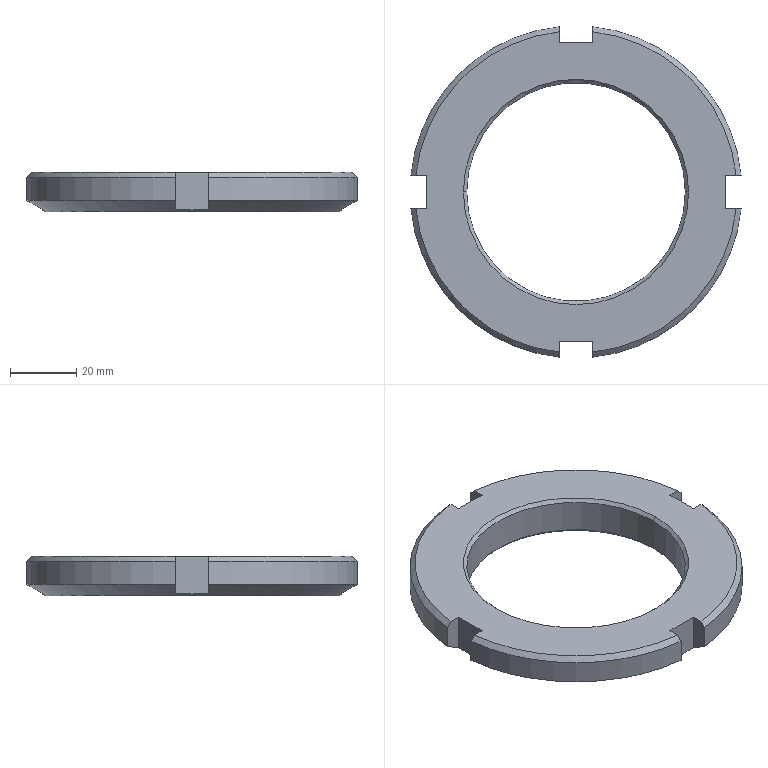Part | SolidWorks | features Chamfer 3, CirPattern 1, Cut 1, Extrusion 1 | 1 solid | 30 faces | box 99.499 x 99.499 x 12 mm | volume 47793 mm3 | plane 14 | cone 10 | cylinder 6 | commonest cylinder face diameters 100 x4 65.835 x2
STEP:
#1=CARTESIAN_POINT('',(-32.917,0.,11.));
#2=VERTEX_POINT('',#1);
#3=CARTESIAN_POINT('',(32.917,0.,11.));
#4=VERTEX_POINT('',#3);
#5=CARTESIAN_POINT('',(0.,0.,11.));
#6=DIRECTION('',(0.,0.,1.));
#7=DIRECTION('',(1.,0.,0.));
#8=AXIS2_PLACEMENT_3D('',#5,#6,#7);
#9=CIRCLE('',#8,32.917);
#10=EDGE_CURVE('',#2,#4,#9,.T.);
#11=ORIENTED_EDGE('',*,*,#10,.F.);
#12=CARTESIAN_POINT('',(-33.918,0.,12.));
#13=VERTEX_POINT('',#12);
#14=CARTESIAN_POINT('',(-32.917,0.,11.));
#15=DIRECTION('',(-0.7071,0.,0.7071));
#16=VECTOR('',#15,1000.);
#17=LINE('',#14,#16);
#18=EDGE_CURVE('',#2,#13,#17,.T.);
#19=ORIENTED_EDGE('',*,*,#18,.T.);
#20=CARTESIAN_POINT('',(33.918,0.,12.));
#21=VERTEX_POINT('',#20);
#22=CARTESIAN_POINT('',(0.,0.,12.));
#23=DIRECTION('',(0.,0.,-1.));
#24=DIRECTION('',(1.,0.,0.));
#25=AXIS2_PLACEMENT_3D('',#22,#23,#24);
#26=CIRCLE('',#25,33.918);
#27=EDGE_CURVE('',#21,#13,#26,.T.);
#28=ORIENTED_EDGE('',*,*,#27,.F.);
#29=CARTESIAN_POINT('',(32.917,0.,11.));
#30=DIRECTION('',(0.7071,0.,0.7071));
#31=VECTOR('',#30,1000.);
#32=LINE('',#29,#31);
#33=EDGE_CURVE('',#4,#21,#32,.T.);
#34=ORIENTED_EDGE('',*,*,#33,.F.);
#35=EDGE_LOOP('',(#11,#19,#28,#34));
#36=FACE_OUTER_BOUND('',#35,.T.);
#37=CARTESIAN_POINT('',(0.,0.,11.));
#38=DIRECTION('',(0.,0.,1.));
#39=DIRECTION('',(1.,0.,0.));
#40=AXIS2_PLACEMENT_3D('',#37,#38,#39);
#41=CONICAL_SURFACE('',#40,32.917,0.7854);
#42=ADVANCED_FACE('',(#36),#41,.F.);
#43=CARTESIAN_POINT('',(32.917,0.,1.));
#44=VERTEX_POINT('',#43);
#45=CARTESIAN_POINT('',(-32.917,0.,1.));
#46=VERTEX_POINT('',#45);
#47=CARTESIAN_POINT('',(0.,0.,1.));
#48=DIRECTION('',(0.,0.,-1.));
#49=DIRECTION('',(1.,0.,0.));
#50=AXIS2_PLACEMENT_3D('',#47,#48,#49);
#51=CIRCLE('',#50,32.917);
#52=EDGE_CURVE('',#44,#46,#51,.T.);
#53=ORIENTED_EDGE('',*,*,#52,.F.);
#54=CARTESIAN_POINT('',(33.918,0.,0.));
#55=VERTEX_POINT('',#54);
#56=CARTESIAN_POINT('',(33.918,0.,0.));
#57=DIRECTION('',(0.7071,0.,-0.7071));
#58=VECTOR('',#57,1000.);
#59=LINE('',#56,#58);
#60=EDGE_CURVE('',#44,#55,#59,.T.);
#61=ORIENTED_EDGE('',*,*,#60,.T.);
#62=CARTESIAN_POINT('',(-33.918,0.,0.));
#63=VERTEX_POINT('',#62);
#64=CARTESIAN_POINT('',(0.,0.,0.));
#65=DIRECTION('',(0.,0.,1.));
#66=DIRECTION('',(1.,0.,0.));
#67=AXIS2_PLACEMENT_3D('',#64,#65,#66);
#68=CIRCLE('',#67,33.918);
#69=EDGE_CURVE('',#63,#55,#68,.T.);
#70=ORIENTED_EDGE('',*,*,#69,.F.);
#71=CARTESIAN_POINT('',(-33.918,0.,0.));
#72=DIRECTION('',(-0.7071,0.,-0.7071));
#73=VECTOR('',#72,1000.);
#74=LINE('',#71,#73);
#75=EDGE_CURVE('',#46,#63,#74,.T.);
#76=ORIENTED_EDGE('',*,*,#75,.F.);
#77=EDGE_LOOP('',(#53,#61,#70,#76));
#78=FACE_OUTER_BOUND('',#77,.T.);
#79=CARTESIAN_POINT('',(0.,0.,0.));
#80=DIRECTION('',(0.,0.,-1.));
#81=DIRECTION('',(-1.,0.,0.));
#82=AXIS2_PLACEMENT_3D('',#79,#80,#81);
#83=CONICAL_SURFACE('',#82,33.918,0.7854);
#84=ADVANCED_FACE('',(#78),#83,.F.);
#85=CARTESIAN_POINT('',(-44.,0.,0.));
#86=VERTEX_POINT('',#85);
#87=CARTESIAN_POINT('',(44.,0.,0.));
#88=VERTEX_POINT('',#87);
#89=CARTESIAN_POINT('',(0.,0.,0.));
#90=DIRECTION('',(0.,0.,-1.));
#91=DIRECTION('',(1.,0.,0.));
#92=AXIS2_PLACEMENT_3D('',#89,#90,#91);
#93=CIRCLE('',#92,44.);
#94=EDGE_CURVE('',#86,#88,#93,.T.);
#95=ORIENTED_EDGE('',*,*,#94,.F.);
#96=CARTESIAN_POINT('',(-44.999,0.,0.577));
#97=VERTEX_POINT('',#96);
#98=CARTESIAN_POINT('',(-50.,0.,3.464));
#99=DIRECTION('',(-0.866,0.,0.5));
#100=VECTOR('',#99,1000.);
#101=LINE('',#98,#100);
#102=EDGE_CURVE('',#86,#97,#101,.T.);
#103=ORIENTED_EDGE('',*,*,#102,.T.);
#104=CARTESIAN_POINT('',(-44.999,5.,0.7369));
#105=VERTEX_POINT('',#104);
#106=CARTESIAN_POINT('',(-44.999,5.,0.7369));
#107=CARTESIAN_POINT('',(-44.999,3.338,0.6309));
#108=CARTESIAN_POINT('',(-44.999,1.671,0.577));
#109=CARTESIAN_POINT('',(-44.999,0.,0.577));
#110=B_SPLINE_CURVE_WITH_KNOTS('',3,(#106,#107,#108,#109),.UNSPECIFIED.,.F.,.F.,(4,4),(0.01219,0.01718),.UNSPECIFIED.);
#111=EDGE_CURVE('',#105,#97,#110,.T.);
#112=ORIENTED_EDGE('',*,*,#111,.F.);
#113=CARTESIAN_POINT('',(-49.749,5.,3.464));
#114=VERTEX_POINT('',#113);
#115=CARTESIAN_POINT('',(-49.749,5.,3.464));
#116=CARTESIAN_POINT('',(-49.476,5.,3.307));
#117=CARTESIAN_POINT('',(-49.202,5.,3.15));
#118=CARTESIAN_POINT('',(-48.929,5.,2.993));
#119=CARTESIAN_POINT('',(-47.619,5.,2.241));
#120=CARTESIAN_POINT('',(-46.309,5.,1.489));
#121=CARTESIAN_POINT('',(-44.999,5.,0.7369));
#122=B_SPLINE_CURVE_WITH_KNOTS('',3,(#115,#116,#117,#118,#119,#120,#121),.UNSPECIFIED.,.F.,.F.,(4,3,4),(0.01027,0.01122,0.01575),.UNSPECIFIED.);
#123=EDGE_CURVE('',#114,#105,#122,.T.);
#124=ORIENTED_EDGE('',*,*,#123,.F.);
#125=CARTESIAN_POINT('',(-5.,49.749,3.464));
#126=VERTEX_POINT('',#125);
#127=CARTESIAN_POINT('',(0.,0.,3.464));
#128=DIRECTION('',(0.,0.,1.));
#129=DIRECTION('',(1.,0.,0.));
#130=AXIS2_PLACEMENT_3D('',#127,#128,#129);
#131=CIRCLE('',#130,50.);
#132=EDGE_CURVE('',#126,#114,#131,.T.);
#133=ORIENTED_EDGE('',*,*,#132,.F.);
#134=CARTESIAN_POINT('',(-5.,44.999,0.7369));
#135=VERTEX_POINT('',#134);
#136=CARTESIAN_POINT('',(-5.,44.999,0.7369));
#137=CARTESIAN_POINT('',(-5.,45.167,0.833));
#138=CARTESIAN_POINT('',(-5.,45.334,0.9291));
#139=CARTESIAN_POINT('',(-5.,45.502,1.025));
#140=CARTESIAN_POINT('',(-5.,46.918,1.838));
#141=CARTESIAN_POINT('',(-5.,48.334,2.651));
#142=CARTESIAN_POINT('',(-5.,49.749,3.464));
#143=B_SPLINE_CURVE_WITH_KNOTS('',3,(#136,#137,#138,#139,#140,#141,#142),.UNSPECIFIED.,.F.,.F.,(4,3,4),(0.01064,0.01122,0.01612),.UNSPECIFIED.);
#144=EDGE_CURVE('',#135,#126,#143,.T.);
#145=ORIENTED_EDGE('',*,*,#144,.F.);
#146=CARTESIAN_POINT('',(5.,44.999,0.7369));
#147=VERTEX_POINT('',#146);
#148=CARTESIAN_POINT('',(5.,44.999,0.7369));
#149=CARTESIAN_POINT('',(3.342,44.999,0.6311));
#150=CARTESIAN_POINT('',(1.679,44.999,0.5772));
#151=CARTESIAN_POINT('',(-0.8215,44.999,0.5769));
#152=CARTESIAN_POINT('',(-1.656,44.999,0.5901));
#153=CARTESIAN_POINT('',(-3.328,44.999,0.6435));
#154=CARTESIAN_POINT('',(-4.165,44.999,0.6837));
#155=CARTESIAN_POINT('',(-5.,44.999,0.7369));
#156=B_SPLINE_CURVE_WITH_KNOTS('',3,(#148,#149,#150,#151,#152,#153,#154,#155),.UNSPECIFIED.,.F.,.F.,(4,2,2,4),(0.01219,0.01717,0.01966,0.02215),.UNSPECIFIED.);
#157=EDGE_CURVE('',#147,#135,#156,.T.);
#158=ORIENTED_EDGE('',*,*,#157,.F.);
#159=CARTESIAN_POINT('',(5.,49.749,3.464));
#160=VERTEX_POINT('',#159);
#161=CARTESIAN_POINT('',(5.,49.749,3.464));
#162=CARTESIAN_POINT('',(5.,48.334,2.651));
#163=CARTESIAN_POINT('',(5.,46.918,1.838));
#164=CARTESIAN_POINT('',(5.,45.502,1.025));
#165=CARTESIAN_POINT('',(5.,45.334,0.9291));
#166=CARTESIAN_POINT('',(5.,45.167,0.833));
#167=CARTESIAN_POINT('',(5.,44.999,0.7369));
#168=B_SPLINE_CURVE_WITH_KNOTS('',3,(#161,#162,#163,#164,#165,#166,#167),.UNSPECIFIED.,.F.,.F.,(4,3,4),(0.006321,0.01122,0.0118),.UNSPECIFIED.);
#169=EDGE_CURVE('',#160,#147,#168,.T.);
#170=ORIENTED_EDGE('',*,*,#169,.F.);
#171=CARTESIAN_POINT('',(49.749,5.,3.464));
#172=VERTEX_POINT('',#171);
#173=CARTESIAN_POINT('',(0.,0.,3.464));
#174=DIRECTION('',(0.,0.,1.));
#175=DIRECTION('',(1.,0.,0.));
#176=AXIS2_PLACEMENT_3D('',#173,#174,#175);
#177=CIRCLE('',#176,50.);
#178=EDGE_CURVE('',#172,#160,#177,.T.);
#179=ORIENTED_EDGE('',*,*,#178,.F.);
#180=CARTESIAN_POINT('',(44.999,5.,0.7369));
#181=VERTEX_POINT('',#180);
#182=CARTESIAN_POINT('',(44.999,5.,0.7369));
#183=CARTESIAN_POINT('',(45.167,5.,0.833));
#184=CARTESIAN_POINT('',(45.334,5.,0.9291));
#185=CARTESIAN_POINT('',(45.502,5.,1.025));
#186=CARTESIAN_POINT('',(46.918,5.,1.838));
#187=CARTESIAN_POINT('',(48.334,5.,2.651));
#188=CARTESIAN_POINT('',(49.749,5.,3.464));
#189=B_SPLINE_CURVE_WITH_KNOTS('',3,(#182,#183,#184,#185,#186,#187,#188),.UNSPECIFIED.,.F.,.F.,(4,3,4),(0.01064,0.01122,0.01612),.UNSPECIFIED.);
#190=EDGE_CURVE('',#181,#172,#189,.T.);
#191=ORIENTED_EDGE('',*,*,#190,.F.);
#192=CARTESIAN_POINT('',(44.999,0.,0.577));
#193=VERTEX_POINT('',#192);
#194=CARTESIAN_POINT('',(44.999,0.,0.577));
#195=CARTESIAN_POINT('',(44.999,1.671,0.577));
#196=CARTESIAN_POINT('',(44.999,3.338,0.6309));
#197=CARTESIAN_POINT('',(44.999,5.,0.7369));
#198=B_SPLINE_CURVE_WITH_KNOTS('',3,(#194,#195,#196,#197),.UNSPECIFIED.,.F.,.F.,(4,4),(0.02472,0.02972),.UNSPECIFIED.);
#199=EDGE_CURVE('',#193,#181,#198,.T.);
#200=ORIENTED_EDGE('',*,*,#199,.F.);
#201=CARTESIAN_POINT('',(50.,0.,3.464));
#202=DIRECTION('',(0.866,0.,0.5));
#203=VECTOR('',#202,1000.);
#204=LINE('',#201,#203);
#205=EDGE_CURVE('',#88,#193,#204,.T.);
#206=ORIENTED_EDGE('',*,*,#205,.F.);
#207=EDGE_LOOP('',(#95,#103,#112,#124,#133,#145,#158,#170,#179,#191,#200,#206));
#208=FACE_OUTER_BOUND('',#207,.T.);
#209=CARTESIAN_POINT('',(0.,0.,3.464));
#210=DIRECTION('',(0.,0.,1.));
#211=DIRECTION('',(1.,0.,0.));
#212=AXIS2_PLACEMENT_3D('',#209,#210,#211);
#213=CONICAL_SURFACE('',#212,50.,1.047);
#214=ADVANCED_FACE('',(#208),#213,.T.);
#215=ORIENTED_EDGE('',*,*,#10,.T.);
#216=CARTESIAN_POINT('',(32.917,0.,12.));
#217=DIRECTION('',(0.,0.,-1.));
#218=VECTOR('',#217,1000.);
#219=LINE('',#216,#218);
#220=EDGE_CURVE('',#4,#44,#219,.T.);
#221=ORIENTED_EDGE('',*,*,#220,.T.);
#222=ORIENTED_EDGE('',*,*,#52,.T.);
#223=CARTESIAN_POINT('',(-32.917,0.,12.));
#224=DIRECTION('',(0.,0.,-1.));
#225=VECTOR('',#224,1000.);
#226=LINE('',#223,#225);
#227=EDGE_CURVE('',#2,#46,#226,.T.);
#228=ORIENTED_EDGE('',*,*,#227,.F.);
#229=EDGE_LOOP('',(#215,#221,#222,#228));
#230=FACE_OUTER_BOUND('',#229,.T.);
#231=CARTESIAN_POINT('',(0.,0.,12.));
#232=DIRECTION('',(0.,0.,-1.));
#233=DIRECTION('',(-1.,0.,0.));
#234=AXIS2_PLACEMENT_3D('',#231,#232,#233);
#235=CYLINDRICAL_SURFACE('',#234,32.917);
#236=ADVANCED_FACE('',(#230),#235,.F.);
#237=CARTESIAN_POINT('',(5.,49.749,10.5));
#238=VERTEX_POINT('',#237);
#239=CARTESIAN_POINT('',(49.749,5.,10.5));
#240=VERTEX_POINT('',#239);
#241=CARTESIAN_POINT('',(0.,0.,10.5));
#242=DIRECTION('',(0.,0.,-1.));
#243=DIRECTION('',(1.,0.,0.));
#244=AXIS2_PLACEMENT_3D('',#241,#242,#243);
#245=CIRCLE('',#244,50.);
#246=EDGE_CURVE('',#238,#240,#245,.T.);
#247=ORIENTED_EDGE('',*,*,#246,.T.);
#248=CARTESIAN_POINT('',(49.749,5.,0.));
#249=DIRECTION('',(0.,0.,1.));
#250=VECTOR('',#249,1000.);
#251=LINE('',#248,#250);
#252=EDGE_CURVE('',#172,#240,#251,.T.);
#253=ORIENTED_EDGE('',*,*,#252,.F.);
#254=ORIENTED_EDGE('',*,*,#178,.T.);
#255=CARTESIAN_POINT('',(5.,49.749,0.));
#256=DIRECTION('',(0.,0.,1.));
#257=VECTOR('',#256,1000.);
#258=LINE('',#255,#257);
#259=EDGE_CURVE('',#160,#238,#258,.T.);
#260=ORIENTED_EDGE('',*,*,#259,.T.);
#261=EDGE_LOOP('',(#247,#253,#254,#260));
#262=FACE_OUTER_BOUND('',#261,.T.);
#263=CARTESIAN_POINT('',(0.,0.,12.));
#264=DIRECTION('',(0.,0.,-1.));
#265=DIRECTION('',(-1.,0.,0.));
#266=AXIS2_PLACEMENT_3D('',#263,#264,#265);
#267=CYLINDRICAL_SURFACE('',#266,50.);
#268=ADVANCED_FACE('',(#262),#267,.T.);
#269=CARTESIAN_POINT('',(48.242,5.,12.));
#270=VERTEX_POINT('',#269);
#271=CARTESIAN_POINT('',(49.749,5.,10.5));
#272=CARTESIAN_POINT('',(49.326,5.,10.921));
#273=CARTESIAN_POINT('',(48.903,5.,11.343));
#274=CARTESIAN_POINT('',(48.479,5.,11.764));
#275=CARTESIAN_POINT('',(48.4,5.,11.842));
#276=CARTESIAN_POINT('',(48.321,5.,11.921));
#277=CARTESIAN_POINT('',(48.242,5.,12.));
#278=B_SPLINE_CURVE_WITH_KNOTS('',3,(#271,#272,#273,#274,#275,#276,#277),.UNSPECIFIED.,.F.,.F.,(4,3,4),(0.00787,0.009662,0.009997),.UNSPECIFIED.);
#279=EDGE_CURVE('',#240,#270,#278,.T.);
#280=ORIENTED_EDGE('',*,*,#279,.F.);
#281=ORIENTED_EDGE('',*,*,#246,.F.);
#282=CARTESIAN_POINT('',(5.,48.242,12.));
#283=VERTEX_POINT('',#282);
#284=CARTESIAN_POINT('',(5.,48.242,12.));
#285=CARTESIAN_POINT('',(5.,48.321,11.921));
#286=CARTESIAN_POINT('',(5.,48.4,11.842));
#287=CARTESIAN_POINT('',(5.,48.479,11.764));
#288=CARTESIAN_POINT('',(5.,48.903,11.343));
#289=CARTESIAN_POINT('',(5.,49.326,10.921));
#290=CARTESIAN_POINT('',(5.,49.749,10.5));
#291=B_SPLINE_CURVE_WITH_KNOTS('',3,(#284,#285,#286,#287,#288,#289,#290),.UNSPECIFIED.,.F.,.F.,(4,3,4),(0.009327,0.009662,0.01145),.UNSPECIFIED.);
#292=EDGE_CURVE('',#283,#238,#291,.T.);
#293=ORIENTED_EDGE('',*,*,#292,.F.);
#294=CARTESIAN_POINT('',(0.,0.,12.));
#295=DIRECTION('',(0.,0.,1.));
#296=DIRECTION('',(1.,0.,0.));
#297=AXIS2_PLACEMENT_3D('',#294,#295,#296);
#298=CIRCLE('',#297,48.5);
#299=EDGE_CURVE('',#270,#283,#298,.T.);
#300=ORIENTED_EDGE('',*,*,#299,.F.);
#301=EDGE_LOOP('',(#280,#281,#293,#300));
#302=FACE_OUTER_BOUND('',#301,.T.);
#303=CARTESIAN_POINT('',(0.,0.,12.));
#304=DIRECTION('',(0.,0.,-1.));
#305=DIRECTION('',(-1.,0.,0.));
#306=AXIS2_PLACEMENT_3D('',#303,#304,#305);
#307=CONICAL_SURFACE('',#306,48.5,0.7854);
#308=ADVANCED_FACE('',(#302),#307,.T.);
#309=CARTESIAN_POINT('',(-49.749,5.,10.5));
#310=VERTEX_POINT('',#309);
#311=CARTESIAN_POINT('',(-5.,49.749,10.5));
#312=VERTEX_POINT('',#311);
#313=CARTESIAN_POINT('',(0.,0.,10.5));
#314=DIRECTION('',(0.,0.,-1.));
#315=DIRECTION('',(1.,0.,0.));
#316=AXIS2_PLACEMENT_3D('',#313,#314,#315);
#317=CIRCLE('',#316,50.);
#318=EDGE_CURVE('',#310,#312,#317,.T.);
#319=ORIENTED_EDGE('',*,*,#318,.T.);
#320=CARTESIAN_POINT('',(-5.,49.749,0.));
#321=DIRECTION('',(0.,0.,1.));
#322=VECTOR('',#321,1000.);
#323=LINE('',#320,#322);
#324=EDGE_CURVE('',#126,#312,#323,.T.);
#325=ORIENTED_EDGE('',*,*,#324,.F.);
#326=ORIENTED_EDGE('',*,*,#132,.T.);
#327=CARTESIAN_POINT('',(-49.749,5.,0.));
#328=DIRECTION('',(0.,0.,1.));
#329=VECTOR('',#328,1000.);
#330=LINE('',#327,#329);
#331=EDGE_CURVE('',#114,#310,#330,.T.);
#332=ORIENTED_EDGE('',*,*,#331,.T.);
#333=EDGE_LOOP('',(#319,#325,#326,#332));
#334=FACE_OUTER_BOUND('',#333,.T.);
#335=CARTESIAN_POINT('',(0.,0.,12.));
#336=DIRECTION('',(0.,0.,-1.));
#337=DIRECTION('',(-1.,0.,0.));
#338=AXIS2_PLACEMENT_3D('',#335,#336,#337);
#339=CYLINDRICAL_SURFACE('',#338,50.);
#340=ADVANCED_FACE('',(#334),#339,.T.);
#341=CARTESIAN_POINT('',(-5.,48.242,12.));
#342=VERTEX_POINT('',#341);
#343=CARTESIAN_POINT('',(-5.,49.749,10.5));
#344=CARTESIAN_POINT('',(-5.,49.326,10.921));
#345=CARTESIAN_POINT('',(-5.,48.903,11.343));
#346=CARTESIAN_POINT('',(-5.,48.479,11.764));
#347=CARTESIAN_POINT('',(-5.,48.4,11.842));
#348=CARTESIAN_POINT('',(-5.,48.321,11.921));
#349=CARTESIAN_POINT('',(-5.,48.242,12.));
#350=B_SPLINE_CURVE_WITH_KNOTS('',3,(#343,#344,#345,#346,#347,#348,#349),.UNSPECIFIED.,.F.,.F.,(4,3,4),(0.00787,0.009662,0.009997),.UNSPECIFIED.);
#351=EDGE_CURVE('',#312,#342,#350,.T.);
#352=ORIENTED_EDGE('',*,*,#351,.F.);
#353=ORIENTED_EDGE('',*,*,#318,.F.);
#354=CARTESIAN_POINT('',(-48.242,5.,12.));
#355=VERTEX_POINT('',#354);
#356=CARTESIAN_POINT('',(-48.242,5.,12.));
#357=CARTESIAN_POINT('',(-48.52,5.,11.723));
#358=CARTESIAN_POINT('',(-48.798,5.,11.447));
#359=CARTESIAN_POINT('',(-49.076,5.,11.17));
#360=CARTESIAN_POINT('',(-49.3,5.,10.947));
#361=CARTESIAN_POINT('',(-49.525,5.,10.723));
#362=CARTESIAN_POINT('',(-49.749,5.,10.5));
#363=B_SPLINE_CURVE_WITH_KNOTS('',3,(#356,#357,#358,#359,#360,#361,#362),.UNSPECIFIED.,.F.,.F.,(4,3,4),(0.008485,0.009662,0.01061),.UNSPECIFIED.);
#364=EDGE_CURVE('',#355,#310,#363,.T.);
#365=ORIENTED_EDGE('',*,*,#364,.F.);
#366=CARTESIAN_POINT('',(0.,0.,12.));
#367=DIRECTION('',(0.,0.,1.));
#368=DIRECTION('',(1.,0.,0.));
#369=AXIS2_PLACEMENT_3D('',#366,#367,#368);
#370=CIRCLE('',#369,48.5);
#371=EDGE_CURVE('',#342,#355,#370,.T.);
#372=ORIENTED_EDGE('',*,*,#371,.F.);
#373=EDGE_LOOP('',(#352,#353,#365,#372));
#374=FACE_OUTER_BOUND('',#373,.T.);
#375=CARTESIAN_POINT('',(0.,0.,12.));
#376=DIRECTION('',(0.,0.,-1.));
#377=DIRECTION('',(-1.,0.,0.));
#378=AXIS2_PLACEMENT_3D('',#375,#376,#377);
#379=CONICAL_SURFACE('',#378,48.5,0.7854);
#380=ADVANCED_FACE('',(#374),#379,.T.);
#381=CARTESIAN_POINT('',(-5.,-49.749,10.5));
#382=VERTEX_POINT('',#381);
#383=CARTESIAN_POINT('',(-49.749,-5.,10.5));
#384=VERTEX_POINT('',#383);
#385=CARTESIAN_POINT('',(0.,0.,10.5));
#386=DIRECTION('',(0.,0.,-1.));
#387=DIRECTION('',(1.,0.,0.));
#388=AXIS2_PLACEMENT_3D('',#385,#386,#387);
#389=CIRCLE('',#388,50.);
#390=EDGE_CURVE('',#382,#384,#389,.T.);
#391=ORIENTED_EDGE('',*,*,#390,.T.);
#392=CARTESIAN_POINT('',(-49.749,-5.,3.464));
#393=VERTEX_POINT('',#392);
#394=CARTESIAN_POINT('',(-49.749,-5.,0.));
#395=DIRECTION('',(0.,0.,1.));
#396=VECTOR('',#395,1000.);
#397=LINE('',#394,#396);
#398=EDGE_CURVE('',#393,#384,#397,.T.);
#399=ORIENTED_EDGE('',*,*,#398,.F.);
#400=CARTESIAN_POINT('',(-5.,-49.749,3.464));
#401=VERTEX_POINT('',#400);
#402=CARTESIAN_POINT('',(0.,0.,3.464));
#403=DIRECTION('',(0.,0.,1.));
#404=DIRECTION('',(1.,0.,0.));
#405=AXIS2_PLACEMENT_3D('',#402,#403,#404);
#406=CIRCLE('',#405,50.);
#407=EDGE_CURVE('',#393,#401,#406,.T.);
#408=ORIENTED_EDGE('',*,*,#407,.T.);
#409=CARTESIAN_POINT('',(-5.,-49.749,0.));
#410=DIRECTION('',(0.,0.,1.));
#411=VECTOR('',#410,1000.);
#412=LINE('',#409,#411);
#413=EDGE_CURVE('',#401,#382,#412,.T.);
#414=ORIENTED_EDGE('',*,*,#413,.T.);
#415=EDGE_LOOP('',(#391,#399,#408,#414));
#416=FACE_OUTER_BOUND('',#415,.T.);
#417=CARTESIAN_POINT('',(0.,0.,12.));
#418=DIRECTION('',(0.,0.,-1.));
#419=DIRECTION('',(-1.,0.,0.));
#420=AXIS2_PLACEMENT_3D('',#417,#418,#419);
#421=CYLINDRICAL_SURFACE('',#420,50.);
#422=ADVANCED_FACE('',(#416),#421,.T.);
#423=CARTESIAN_POINT('',(-48.242,-5.,12.));
#424=VERTEX_POINT('',#423);
#425=CARTESIAN_POINT('',(-49.749,-5.,10.5));
#426=CARTESIAN_POINT('',(-49.525,-5.,10.723));
#427=CARTESIAN_POINT('',(-49.3,-5.,10.947));
#428=CARTESIAN_POINT('',(-49.076,-5.,11.17));
#429=CARTESIAN_POINT('',(-48.798,-5.,11.447));
#430=CARTESIAN_POINT('',(-48.52,-5.,11.723));
#431=CARTESIAN_POINT('',(-48.242,-5.,12.));
#432=B_SPLINE_CURVE_WITH_KNOTS('',3,(#425,#426,#427,#428,#429,#430,#431),.UNSPECIFIED.,.F.,.F.,(4,3,4),(0.008712,0.009662,0.01084),.UNSPECIFIED.);
#433=EDGE_CURVE('',#384,#424,#432,.T.);
#434=ORIENTED_EDGE('',*,*,#433,.F.);
#435=ORIENTED_EDGE('',*,*,#390,.F.);
#436=CARTESIAN_POINT('',(-5.,-48.242,12.));
#437=VERTEX_POINT('',#436);
#438=CARTESIAN_POINT('',(-5.,-48.242,12.));
#439=CARTESIAN_POINT('',(-5.,-48.52,11.723));
#440=CARTESIAN_POINT('',(-5.,-48.798,11.447));
#441=CARTESIAN_POINT('',(-5.,-49.076,11.17));
#442=CARTESIAN_POINT('',(-5.,-49.3,10.947));
#443=CARTESIAN_POINT('',(-5.,-49.525,10.723));
#444=CARTESIAN_POINT('',(-5.,-49.749,10.5));
#445=B_SPLINE_CURVE_WITH_KNOTS('',3,(#438,#439,#440,#441,#442,#443,#444),.UNSPECIFIED.,.F.,.F.,(4,3,4),(0.008485,0.009662,0.01061),.UNSPECIFIED.);
#446=EDGE_CURVE('',#437,#382,#445,.T.);
#447=ORIENTED_EDGE('',*,*,#446,.F.);
#448=CARTESIAN_POINT('',(0.,0.,12.));
#449=DIRECTION('',(0.,0.,1.));
#450=DIRECTION('',(1.,0.,0.));
#451=AXIS2_PLACEMENT_3D('',#448,#449,#450);
#452=CIRCLE('',#451,48.5);
#453=EDGE_CURVE('',#424,#437,#452,.T.);
#454=ORIENTED_EDGE('',*,*,#453,.F.);
#455=EDGE_LOOP('',(#434,#435,#447,#454));
#456=FACE_OUTER_BOUND('',#455,.T.);
#457=CARTESIAN_POINT('',(0.,0.,12.));
#458=DIRECTION('',(0.,0.,-1.));
#459=DIRECTION('',(-1.,0.,0.));
#460=AXIS2_PLACEMENT_3D('',#457,#458,#459);
#461=CONICAL_SURFACE('',#460,48.5,0.7854);
#462=ADVANCED_FACE('',(#456),#461,.T.);
#463=ORIENTED_EDGE('',*,*,#27,.T.);
#464=CARTESIAN_POINT('',(0.,0.,12.));
#465=DIRECTION('',(0.,0.,-1.));
#466=DIRECTION('',(1.,0.,0.));
#467=AXIS2_PLACEMENT_3D('',#464,#465,#466);
#468=CIRCLE('',#467,33.918);
#469=EDGE_CURVE('',#13,#21,#468,.T.);
#470=ORIENTED_EDGE('',*,*,#469,.T.);
#471=EDGE_LOOP('',(#463,#470));
#472=FACE_BOUND('',#471,.T.);
#473=CARTESIAN_POINT('',(44.999,5.,12.));
#474=VERTEX_POINT('',#473);
#475=CARTESIAN_POINT('',(44.999,5.,12.));
#476=DIRECTION('',(-1.,0.,0.));
#477=VECTOR('',#476,1000.);
#478=LINE('',#475,#477);
#479=EDGE_CURVE('',#270,#474,#478,.T.);
#480=ORIENTED_EDGE('',*,*,#479,.F.);
#481=ORIENTED_EDGE('',*,*,#299,.T.);
#482=CARTESIAN_POINT('',(5.,44.999,12.));
#483=VERTEX_POINT('',#482);
#484=CARTESIAN_POINT('',(5.,44.999,12.));
#485=DIRECTION('',(0.,1.,0.));
#486=VECTOR('',#485,1000.);
#487=LINE('',#484,#486);
#488=EDGE_CURVE('',#483,#283,#487,.T.);
#489=ORIENTED_EDGE('',*,*,#488,.F.);
#490=CARTESIAN_POINT('',(-5.,44.999,12.));
#491=VERTEX_POINT('',#490);
#492=CARTESIAN_POINT('',(5.,44.999,12.));
#493=DIRECTION('',(1.,0.,0.));
#494=VECTOR('',#493,1000.);
#495=LINE('',#492,#494);
#496=EDGE_CURVE('',#491,#483,#495,.T.);
#497=ORIENTED_EDGE('',*,*,#496,.F.);
#498=CARTESIAN_POINT('',(-5.,44.999,12.));
#499=DIRECTION('',(0.,-1.,0.));
#500=VECTOR('',#499,1000.);
#501=LINE('',#498,#500);
#502=EDGE_CURVE('',#342,#491,#501,.T.);
#503=ORIENTED_EDGE('',*,*,#502,.F.);
#504=ORIENTED_EDGE('',*,*,#371,.T.);
#505=CARTESIAN_POINT('',(-44.999,5.,12.));
#506=VERTEX_POINT('',#505);
#507=CARTESIAN_POINT('',(-44.999,5.,12.));
#508=DIRECTION('',(-1.,0.,0.));
#509=VECTOR('',#508,1000.);
#510=LINE('',#507,#509);
#511=EDGE_CURVE('',#506,#355,#510,.T.);
#512=ORIENTED_EDGE('',*,*,#511,.F.);
#513=CARTESIAN_POINT('',(-44.999,-5.,12.));
#514=VERTEX_POINT('',#513);
#515=CARTESIAN_POINT('',(-44.999,5.,12.));
#516=DIRECTION('',(0.,1.,0.));
#517=VECTOR('',#516,1000.);
#518=LINE('',#515,#517);
#519=EDGE_CURVE('',#514,#506,#518,.T.);
#520=ORIENTED_EDGE('',*,*,#519,.F.);
#521=CARTESIAN_POINT('',(-44.999,-5.,12.));
#522=DIRECTION('',(1.,0.,0.));
#523=VECTOR('',#522,1000.);
#524=LINE('',#521,#523);
#525=EDGE_CURVE('',#424,#514,#524,.T.);
#526=ORIENTED_EDGE('',*,*,#525,.F.);
#527=ORIENTED_EDGE('',*,*,#453,.T.);
#528=CARTESIAN_POINT('',(-5.,-44.999,12.));
#529=VERTEX_POINT('',#528);
#530=CARTESIAN_POINT('',(-5.,-44.999,12.));
#531=DIRECTION('',(0.,-1.,0.));
#532=VECTOR('',#531,1000.);
#533=LINE('',#530,#532);
#534=EDGE_CURVE('',#529,#437,#533,.T.);
#535=ORIENTED_EDGE('',*,*,#534,.F.);
#536=CARTESIAN_POINT('',(5.,-44.999,12.));
#537=VERTEX_POINT('',#536);
#538=CARTESIAN_POINT('',(-5.,-44.999,12.));
#539=DIRECTION('',(-1.,0.,0.));
#540=VECTOR('',#539,1000.);
#541=LINE('',#538,#540);
#542=EDGE_CURVE('',#537,#529,#541,.T.);
#543=ORIENTED_EDGE('',*,*,#542,.F.);
#544=CARTESIAN_POINT('',(5.,-48.242,12.));
#545=VERTEX_POINT('',#544);
#546=CARTESIAN_POINT('',(5.,-44.999,12.));
#547=DIRECTION('',(0.,1.,0.));
#548=VECTOR('',#547,1000.);
#549=LINE('',#546,#548);
#550=EDGE_CURVE('',#545,#537,#549,.T.);
#551=ORIENTED_EDGE('',*,*,#550,.F.);
#552=CARTESIAN_POINT('',(48.242,-5.,12.));
#553=VERTEX_POINT('',#552);
#554=CARTESIAN_POINT('',(0.,0.,12.));
#555=DIRECTION('',(0.,0.,1.));
#556=DIRECTION('',(1.,0.,0.));
#557=AXIS2_PLACEMENT_3D('',#554,#555,#556);
#558=CIRCLE('',#557,48.5);
#559=EDGE_CURVE('',#545,#553,#558,.T.);
#560=ORIENTED_EDGE('',*,*,#559,.T.);
#561=CARTESIAN_POINT('',(44.999,-5.,12.));
#562=VERTEX_POINT('',#561);
#563=CARTESIAN_POINT('',(44.999,-5.,12.));
#564=DIRECTION('',(1.,0.,0.));
#565=VECTOR('',#564,1000.);
#566=LINE('',#563,#565);
#567=EDGE_CURVE('',#562,#553,#566,.T.);
#568=ORIENTED_EDGE('',*,*,#567,.F.);
#569=CARTESIAN_POINT('',(44.999,-5.,12.));
#570=DIRECTION('',(0.,-1.,0.));
#571=VECTOR('',#570,1000.);
#572=LINE('',#569,#571);
#573=EDGE_CURVE('',#474,#562,#572,.T.);
#574=ORIENTED_EDGE('',*,*,#573,.F.);
#575=EDGE_LOOP('',(#480,#481,#489,#497,#503,#504,#512,#520,#526,#527,#535,#543,#551,#560,#568,#574));
#576=FACE_OUTER_BOUND('',#575,.T.);
#577=CARTESIAN_POINT('',(0.,0.,12.));
#578=DIRECTION('',(0.,0.,1.));
#579=DIRECTION('',(1.,0.,0.));
#580=AXIS2_PLACEMENT_3D('',#577,#578,#579);
#581=PLANE('',#580);
#582=ADVANCED_FACE('',(#472,#576),#581,.T.);
#583=ORIENTED_EDGE('',*,*,#69,.T.);
#584=CARTESIAN_POINT('',(0.,0.,0.));
#585=DIRECTION('',(0.,0.,1.));
#586=DIRECTION('',(1.,0.,0.));
#587=AXIS2_PLACEMENT_3D('',#584,#585,#586);
#588=CIRCLE('',#587,33.918);
#589=EDGE_CURVE('',#55,#63,#588,.T.);
#590=ORIENTED_EDGE('',*,*,#589,.T.);
#591=EDGE_LOOP('',(#583,#590));
#592=FACE_BOUND('',#591,.T.);
#593=CARTESIAN_POINT('',(0.,0.,0.));
#594=DIRECTION('',(0.,0.,-1.));
#595=DIRECTION('',(1.,0.,0.));
#596=AXIS2_PLACEMENT_3D('',#593,#594,#595);
#597=CIRCLE('',#596,44.);
#598=EDGE_CURVE('',#88,#86,#597,.T.);
#599=ORIENTED_EDGE('',*,*,#598,.T.);
#600=ORIENTED_EDGE('',*,*,#94,.T.);
#601=EDGE_LOOP('',(#599,#600));
#602=FACE_OUTER_BOUND('',#601,.T.);
#603=CARTESIAN_POINT('',(0.,0.,0.));
#604=DIRECTION('',(0.,0.,1.));
#605=DIRECTION('',(1.,0.,0.));
#606=AXIS2_PLACEMENT_3D('',#603,#604,#605);
#607=PLANE('',#606);
#608=ADVANCED_FACE('',(#592,#602),#607,.F.);
#609=CARTESIAN_POINT('',(5.,-49.749,3.464));
#610=VERTEX_POINT('',#609);
#611=CARTESIAN_POINT('',(49.749,-5.,3.464));
#612=VERTEX_POINT('',#611);
#613=CARTESIAN_POINT('',(0.,0.,3.464));
#614=DIRECTION('',(0.,0.,1.));
#615=DIRECTION('',(1.,0.,0.));
#616=AXIS2_PLACEMENT_3D('',#613,#614,#615);
#617=CIRCLE('',#616,50.);
#618=EDGE_CURVE('',#610,#612,#617,.T.);
#619=ORIENTED_EDGE('',*,*,#618,.T.);
#620=CARTESIAN_POINT('',(49.749,-5.,10.5));
#621=VERTEX_POINT('',#620);
#622=CARTESIAN_POINT('',(49.749,-5.,0.));
#623=DIRECTION('',(0.,0.,1.));
#624=VECTOR('',#623,1000.);
#625=LINE('',#622,#624);
#626=EDGE_CURVE('',#612,#621,#625,.T.);
#627=ORIENTED_EDGE('',*,*,#626,.T.);
#628=CARTESIAN_POINT('',(5.,-49.749,10.5));
#629=VERTEX_POINT('',#628);
#630=CARTESIAN_POINT('',(0.,0.,10.5));
#631=DIRECTION('',(0.,0.,-1.));
#632=DIRECTION('',(1.,0.,0.));
#633=AXIS2_PLACEMENT_3D('',#630,#631,#632);
#634=CIRCLE('',#633,50.);
#635=EDGE_CURVE('',#621,#629,#634,.T.);
#636=ORIENTED_EDGE('',*,*,#635,.T.);
#637=CARTESIAN_POINT('',(5.,-49.749,0.));
#638=DIRECTION('',(0.,0.,1.));
#639=VECTOR('',#638,1000.);
#640=LINE('',#637,#639);
#641=EDGE_CURVE('',#610,#629,#640,.T.);
#642=ORIENTED_EDGE('',*,*,#641,.F.);
#643=EDGE_LOOP('',(#619,#627,#636,#642));
#644=FACE_OUTER_BOUND('',#643,.T.);
#645=CARTESIAN_POINT('',(0.,0.,12.));
#646=DIRECTION('',(0.,0.,-1.));
#647=DIRECTION('',(-1.,0.,0.));
#648=AXIS2_PLACEMENT_3D('',#645,#646,#647);
#649=CYLINDRICAL_SURFACE('',#648,50.);
#650=ADVANCED_FACE('',(#644),#649,.T.);
#651=ORIENTED_EDGE('',*,*,#220,.F.);
#652=CARTESIAN_POINT('',(0.,0.,11.));
#653=DIRECTION('',(0.,0.,1.));
#654=DIRECTION('',(1.,0.,0.));
#655=AXIS2_PLACEMENT_3D('',#652,#653,#654);
#656=CIRCLE('',#655,32.917);
#657=EDGE_CURVE('',#4,#2,#656,.T.);
#658=ORIENTED_EDGE('',*,*,#657,.T.);
#659=ORIENTED_EDGE('',*,*,#227,.T.);
#660=CARTESIAN_POINT('',(0.,0.,1.));
#661=DIRECTION('',(0.,0.,-1.));
#662=DIRECTION('',(1.,0.,0.));
#663=AXIS2_PLACEMENT_3D('',#660,#661,#662);
#664=CIRCLE('',#663,32.917);
#665=EDGE_CURVE('',#46,#44,#664,.T.);
#666=ORIENTED_EDGE('',*,*,#665,.T.);
#667=EDGE_LOOP('',(#651,#658,#659,#666));
#668=FACE_OUTER_BOUND('',#667,.T.);
#669=CARTESIAN_POINT('',(0.,0.,12.));
#670=DIRECTION('',(0.,0.,-1.));
#671=DIRECTION('',(-1.,0.,0.));
#672=AXIS2_PLACEMENT_3D('',#669,#670,#671);
#673=CYLINDRICAL_SURFACE('',#672,32.917);
#674=ADVANCED_FACE('',(#668),#673,.F.);
#675=CARTESIAN_POINT('',(48.242,-5.,12.));
#676=CARTESIAN_POINT('',(48.321,-5.,11.921));
#677=CARTESIAN_POINT('',(48.4,-5.,11.842));
#678=CARTESIAN_POINT('',(48.479,-5.,11.764));
#679=CARTESIAN_POINT('',(48.903,-5.,11.343));
#680=CARTESIAN_POINT('',(49.326,-5.,10.921));
#681=CARTESIAN_POINT('',(49.749,-5.,10.5));
#682=B_SPLINE_CURVE_WITH_KNOTS('',3,(#675,#676,#677,#678,#679,#680,#681),.UNSPECIFIED.,.F.,.F.,(4,3,4),(0.009327,0.009662,0.01145),.UNSPECIFIED.);
#683=EDGE_CURVE('',#553,#621,#682,.T.);
#684=ORIENTED_EDGE('',*,*,#683,.F.);
#685=ORIENTED_EDGE('',*,*,#559,.F.);
#686=CARTESIAN_POINT('',(5.,-49.749,10.5));
#687=CARTESIAN_POINT('',(5.,-49.525,10.723));
#688=CARTESIAN_POINT('',(5.,-49.3,10.947));
#689=CARTESIAN_POINT('',(5.,-49.076,11.17));
#690=CARTESIAN_POINT('',(5.,-48.798,11.447));
#691=CARTESIAN_POINT('',(5.,-48.52,11.723));
#692=CARTESIAN_POINT('',(5.,-48.242,12.));
#693=B_SPLINE_CURVE_WITH_KNOTS('',3,(#686,#687,#688,#689,#690,#691,#692),.UNSPECIFIED.,.F.,.F.,(4,3,4),(0.008712,0.009662,0.01084),.UNSPECIFIED.);
#694=EDGE_CURVE('',#629,#545,#693,.T.);
#695=ORIENTED_EDGE('',*,*,#694,.F.);
#696=ORIENTED_EDGE('',*,*,#635,.F.);
#697=EDGE_LOOP('',(#684,#685,#695,#696));
#698=FACE_OUTER_BOUND('',#697,.T.);
#699=CARTESIAN_POINT('',(0.,0.,12.));
#700=DIRECTION('',(0.,0.,-1.));
#701=DIRECTION('',(-1.,0.,0.));
#702=AXIS2_PLACEMENT_3D('',#699,#700,#701);
#703=CONICAL_SURFACE('',#702,48.5,0.7854);
#704=ADVANCED_FACE('',(#698),#703,.T.);
#705=ORIENTED_EDGE('',*,*,#102,.F.);
#706=ORIENTED_EDGE('',*,*,#598,.F.);
#707=ORIENTED_EDGE('',*,*,#205,.T.);
#708=CARTESIAN_POINT('',(44.999,-5.,0.7369));
#709=VERTEX_POINT('',#708);
#710=CARTESIAN_POINT('',(44.999,-5.,0.7369));
#711=CARTESIAN_POINT('',(44.999,-4.167,0.6838));
#712=CARTESIAN_POINT('',(44.999,-3.332,0.6437));
#713=CARTESIAN_POINT('',(44.999,-1.664,0.5903));
#714=CARTESIAN_POINT('',(44.999,-0.8315,0.577));
#715=CARTESIAN_POINT('',(44.999,0.,0.577));
#716=B_SPLINE_CURVE_WITH_KNOTS('',3,(#710,#711,#712,#713,#714,#715),.UNSPECIFIED.,.F.,.F.,(4,2,4),(0.01974,0.02223,0.02472),.UNSPECIFIED.);
#717=EDGE_CURVE('',#709,#193,#716,.T.);
#718=ORIENTED_EDGE('',*,*,#717,.F.);
#719=CARTESIAN_POINT('',(49.749,-5.,3.464));
#720=CARTESIAN_POINT('',(48.334,-5.,2.651));
#721=CARTESIAN_POINT('',(46.918,-5.,1.838));
#722=CARTESIAN_POINT('',(45.502,-5.,1.025));
#723=CARTESIAN_POINT('',(45.334,-5.,0.9291));
#724=CARTESIAN_POINT('',(45.167,-5.,0.833));
#725=CARTESIAN_POINT('',(44.999,-5.,0.7369));
#726=B_SPLINE_CURVE_WITH_KNOTS('',3,(#719,#720,#721,#722,#723,#724,#725),.UNSPECIFIED.,.F.,.F.,(4,3,4),(0.006321,0.01122,0.0118),.UNSPECIFIED.);
#727=EDGE_CURVE('',#612,#709,#726,.T.);
#728=ORIENTED_EDGE('',*,*,#727,.F.);
#729=ORIENTED_EDGE('',*,*,#618,.F.);
#730=CARTESIAN_POINT('',(5.,-44.999,0.7369));
#731=VERTEX_POINT('',#730);
#732=CARTESIAN_POINT('',(5.,-44.999,0.7369));
#733=CARTESIAN_POINT('',(5.,-46.309,1.489));
#734=CARTESIAN_POINT('',(5.,-47.619,2.241));
#735=CARTESIAN_POINT('',(5.,-48.929,2.993));
#736=CARTESIAN_POINT('',(5.,-49.202,3.15));
#737=CARTESIAN_POINT('',(5.,-49.476,3.307));
#738=CARTESIAN_POINT('',(5.,-49.749,3.464));
#739=B_SPLINE_CURVE_WITH_KNOTS('',3,(#732,#733,#734,#735,#736,#737,#738),.UNSPECIFIED.,.F.,.F.,(4,3,4),(0.006688,0.01122,0.01217),.UNSPECIFIED.);
#740=EDGE_CURVE('',#731,#610,#739,.T.);
#741=ORIENTED_EDGE('',*,*,#740,.F.);
#742=CARTESIAN_POINT('',(-5.,-44.999,0.7369));
#743=VERTEX_POINT('',#742);
#744=CARTESIAN_POINT('',(-5.,-44.999,0.7369));
#745=CARTESIAN_POINT('',(-4.165,-44.999,0.6837));
#746=CARTESIAN_POINT('',(-3.328,-44.999,0.6435));
#747=CARTESIAN_POINT('',(-1.656,-44.999,0.5901));
#748=CARTESIAN_POINT('',(-0.8215,-44.999,0.5769));
#749=CARTESIAN_POINT('',(1.679,-44.999,0.5772));
#750=CARTESIAN_POINT('',(3.342,-44.999,0.6311));
#751=CARTESIAN_POINT('',(5.,-44.999,0.7369));
#752=B_SPLINE_CURVE_WITH_KNOTS('',3,(#744,#745,#746,#747,#748,#749,#750,#751),.UNSPECIFIED.,.F.,.F.,(4,2,2,4),(0.01974,0.02224,0.02473,0.02972),.UNSPECIFIED.);
#753=EDGE_CURVE('',#743,#731,#752,.T.);
#754=ORIENTED_EDGE('',*,*,#753,.F.);
#755=CARTESIAN_POINT('',(-5.,-49.749,3.464));
#756=CARTESIAN_POINT('',(-5.,-49.476,3.307));
#757=CARTESIAN_POINT('',(-5.,-49.202,3.15));
#758=CARTESIAN_POINT('',(-5.,-48.929,2.993));
#759=CARTESIAN_POINT('',(-5.,-47.619,2.241));
#760=CARTESIAN_POINT('',(-5.,-46.309,1.489));
#761=CARTESIAN_POINT('',(-5.,-44.999,0.7369));
#762=B_SPLINE_CURVE_WITH_KNOTS('',3,(#755,#756,#757,#758,#759,#760,#761),.UNSPECIFIED.,.F.,.F.,(4,3,4),(0.01027,0.01122,0.01575),.UNSPECIFIED.);
#763=EDGE_CURVE('',#401,#743,#762,.T.);
#764=ORIENTED_EDGE('',*,*,#763,.F.);
#765=ORIENTED_EDGE('',*,*,#407,.F.);
#766=CARTESIAN_POINT('',(-44.999,-5.,0.7369));
#767=VERTEX_POINT('',#766);
#768=CARTESIAN_POINT('',(-44.999,-5.,0.7369));
#769=CARTESIAN_POINT('',(-46.309,-5.,1.489));
#770=CARTESIAN_POINT('',(-47.619,-5.,2.241));
#771=CARTESIAN_POINT('',(-48.929,-5.,2.993));
#772=CARTESIAN_POINT('',(-49.202,-5.,3.15));
#773=CARTESIAN_POINT('',(-49.476,-5.,3.307));
#774=CARTESIAN_POINT('',(-49.749,-5.,3.464));
#775=B_SPLINE_CURVE_WITH_KNOTS('',3,(#768,#769,#770,#771,#772,#773,#774),.UNSPECIFIED.,.F.,.F.,(4,3,4),(0.006688,0.01122,0.01217),.UNSPECIFIED.);
#776=EDGE_CURVE('',#767,#393,#775,.T.);
#777=ORIENTED_EDGE('',*,*,#776,.F.);
#778=CARTESIAN_POINT('',(-44.999,0.,0.577));
#779=CARTESIAN_POINT('',(-44.999,-0.8315,0.577));
#780=CARTESIAN_POINT('',(-44.999,-1.664,0.5903));
#781=CARTESIAN_POINT('',(-44.999,-3.332,0.6437));
#782=CARTESIAN_POINT('',(-44.999,-4.167,0.6838));
#783=CARTESIAN_POINT('',(-44.999,-5.,0.7369));
#784=B_SPLINE_CURVE_WITH_KNOTS('',3,(#778,#779,#780,#781,#782,#783),.UNSPECIFIED.,.F.,.F.,(4,2,4),(0.01718,0.01967,0.02215),.UNSPECIFIED.);
#785=EDGE_CURVE('',#97,#767,#784,.T.);
#786=ORIENTED_EDGE('',*,*,#785,.F.);
#787=EDGE_LOOP('',(#705,#706,#707,#718,#728,#729,#741,#754,#764,#765,#777,#786));
#788=FACE_OUTER_BOUND('',#787,.T.);
#789=CARTESIAN_POINT('',(0.,0.,3.464));
#790=DIRECTION('',(0.,0.,1.));
#791=DIRECTION('',(1.,0.,0.));
#792=AXIS2_PLACEMENT_3D('',#789,#790,#791);
#793=CONICAL_SURFACE('',#792,50.,1.047);
#794=ADVANCED_FACE('',(#788),#793,.T.);
#795=ORIENTED_EDGE('',*,*,#753,.T.);
#796=CARTESIAN_POINT('',(5.,-44.999,0.));
#797=DIRECTION('',(0.,0.,1.));
#798=VECTOR('',#797,1000.);
#799=LINE('',#796,#798);
#800=EDGE_CURVE('',#731,#537,#799,.T.);
#801=ORIENTED_EDGE('',*,*,#800,.T.);
#802=ORIENTED_EDGE('',*,*,#542,.T.);
#803=CARTESIAN_POINT('',(-5.,-44.999,0.));
#804=DIRECTION('',(0.,0.,1.));
#805=VECTOR('',#804,1000.);
#806=LINE('',#803,#805);
#807=EDGE_CURVE('',#743,#529,#806,.T.);
#808=ORIENTED_EDGE('',*,*,#807,.F.);
#809=EDGE_LOOP('',(#795,#801,#802,#808));
#810=FACE_OUTER_BOUND('',#809,.T.);
#811=CARTESIAN_POINT('',(-5.,-44.999,0.));
#812=DIRECTION('',(0.,1.,0.));
#813=DIRECTION('',(0.,0.,1.));
#814=AXIS2_PLACEMENT_3D('',#811,#812,#813);
#815=PLANE('',#814);
#816=ADVANCED_FACE('',(#810),#815,.F.);
#817=ORIENTED_EDGE('',*,*,#694,.T.);
#818=ORIENTED_EDGE('',*,*,#550,.T.);
#819=ORIENTED_EDGE('',*,*,#800,.F.);
#820=ORIENTED_EDGE('',*,*,#740,.T.);
#821=ORIENTED_EDGE('',*,*,#641,.T.);
#822=EDGE_LOOP('',(#817,#818,#819,#820,#821));
#823=FACE_OUTER_BOUND('',#822,.T.);
#824=CARTESIAN_POINT('',(5.,-44.999,0.));
#825=DIRECTION('',(1.,0.,0.));
#826=DIRECTION('',(0.,0.,-1.));
#827=AXIS2_PLACEMENT_3D('',#824,#825,#826);
#828=PLANE('',#827);
#829=ADVANCED_FACE('',(#823),#828,.F.);
#830=ORIENTED_EDGE('',*,*,#446,.T.);
#831=ORIENTED_EDGE('',*,*,#413,.F.);
#832=ORIENTED_EDGE('',*,*,#763,.T.);
#833=ORIENTED_EDGE('',*,*,#807,.T.);
#834=ORIENTED_EDGE('',*,*,#534,.T.);
#835=EDGE_LOOP('',(#830,#831,#832,#833,#834));
#836=FACE_OUTER_BOUND('',#835,.T.);
#837=CARTESIAN_POINT('',(-5.,-44.999,0.));
#838=DIRECTION('',(-1.,0.,0.));
#839=DIRECTION('',(0.,0.,1.));
#840=AXIS2_PLACEMENT_3D('',#837,#838,#839);
#841=PLANE('',#840);
#842=ADVANCED_FACE('',(#836),#841,.F.);
#843=ORIENTED_EDGE('',*,*,#111,.T.);
#844=ORIENTED_EDGE('',*,*,#785,.T.);
#845=CARTESIAN_POINT('',(-44.999,-5.,0.));
#846=DIRECTION('',(0.,0.,1.));
#847=VECTOR('',#846,1000.);
#848=LINE('',#845,#847);
#849=EDGE_CURVE('',#767,#514,#848,.T.);
#850=ORIENTED_EDGE('',*,*,#849,.T.);
#851=ORIENTED_EDGE('',*,*,#519,.T.);
#852=CARTESIAN_POINT('',(-44.999,5.,0.));
#853=DIRECTION('',(0.,0.,1.));
#854=VECTOR('',#853,1000.);
#855=LINE('',#852,#854);
#856=EDGE_CURVE('',#105,#506,#855,.T.);
#857=ORIENTED_EDGE('',*,*,#856,.F.);
#858=EDGE_LOOP('',(#843,#844,#850,#851,#857));
#859=FACE_OUTER_BOUND('',#858,.T.);
#860=CARTESIAN_POINT('',(-44.999,5.,0.));
#861=DIRECTION('',(1.,0.,0.));
#862=DIRECTION('',(0.,1.,0.));
#863=AXIS2_PLACEMENT_3D('',#860,#861,#862);
#864=PLANE('',#863);
#865=ADVANCED_FACE('',(#859),#864,.F.);
#866=ORIENTED_EDGE('',*,*,#433,.T.);
#867=ORIENTED_EDGE('',*,*,#525,.T.);
#868=ORIENTED_EDGE('',*,*,#849,.F.);
#869=ORIENTED_EDGE('',*,*,#776,.T.);
#870=ORIENTED_EDGE('',*,*,#398,.T.);
#871=EDGE_LOOP('',(#866,#867,#868,#869,#870));
#872=FACE_OUTER_BOUND('',#871,.T.);
#873=CARTESIAN_POINT('',(-44.999,-5.,0.));
#874=DIRECTION('',(0.,-1.,0.));
#875=DIRECTION('',(1.,0.,0.));
#876=AXIS2_PLACEMENT_3D('',#873,#874,#875);
#877=PLANE('',#876);
#878=ADVANCED_FACE('',(#872),#877,.F.);
#879=ORIENTED_EDGE('',*,*,#364,.T.);
#880=ORIENTED_EDGE('',*,*,#331,.F.);
#881=ORIENTED_EDGE('',*,*,#123,.T.);
#882=ORIENTED_EDGE('',*,*,#856,.T.);
#883=ORIENTED_EDGE('',*,*,#511,.T.);
#884=EDGE_LOOP('',(#879,#880,#881,#882,#883));
#885=FACE_OUTER_BOUND('',#884,.T.);
#886=CARTESIAN_POINT('',(-44.999,5.,0.));
#887=DIRECTION('',(0.,1.,0.));
#888=DIRECTION('',(-1.,0.,0.));
#889=AXIS2_PLACEMENT_3D('',#886,#887,#888);
#890=PLANE('',#889);
#891=ADVANCED_FACE('',(#885),#890,.F.);
#892=ORIENTED_EDGE('',*,*,#157,.T.);
#893=CARTESIAN_POINT('',(-5.,44.999,0.));
#894=DIRECTION('',(0.,0.,1.));
#895=VECTOR('',#894,1000.);
#896=LINE('',#893,#895);
#897=EDGE_CURVE('',#135,#491,#896,.T.);
#898=ORIENTED_EDGE('',*,*,#897,.T.);
#899=ORIENTED_EDGE('',*,*,#496,.T.);
#900=CARTESIAN_POINT('',(5.,44.999,0.));
#901=DIRECTION('',(0.,0.,1.));
#902=VECTOR('',#901,1000.);
#903=LINE('',#900,#902);
#904=EDGE_CURVE('',#147,#483,#903,.T.);
#905=ORIENTED_EDGE('',*,*,#904,.F.);
#906=EDGE_LOOP('',(#892,#898,#899,#905));
#907=FACE_OUTER_BOUND('',#906,.T.);
#908=CARTESIAN_POINT('',(5.,44.999,0.));
#909=DIRECTION('',(0.,-1.,0.));
#910=DIRECTION('',(1.,0.,0.));
#911=AXIS2_PLACEMENT_3D('',#908,#909,#910);
#912=PLANE('',#911);
#913=ADVANCED_FACE('',(#907),#912,.F.);
#914=ORIENTED_EDGE('',*,*,#351,.T.);
#915=ORIENTED_EDGE('',*,*,#502,.T.);
#916=ORIENTED_EDGE('',*,*,#897,.F.);
#917=ORIENTED_EDGE('',*,*,#144,.T.);
#918=ORIENTED_EDGE('',*,*,#324,.T.);
#919=EDGE_LOOP('',(#914,#915,#916,#917,#918));
#920=FACE_OUTER_BOUND('',#919,.T.);
#921=CARTESIAN_POINT('',(-5.,44.999,0.));
#922=DIRECTION('',(-1.,0.,0.));
#923=DIRECTION('',(0.,-1.,0.));
#924=AXIS2_PLACEMENT_3D('',#921,#922,#923);
#925=PLANE('',#924);
#926=ADVANCED_FACE('',(#920),#925,.F.);
#927=ORIENTED_EDGE('',*,*,#292,.T.);
#928=ORIENTED_EDGE('',*,*,#259,.F.);
#929=ORIENTED_EDGE('',*,*,#169,.T.);
#930=ORIENTED_EDGE('',*,*,#904,.T.);
#931=ORIENTED_EDGE('',*,*,#488,.T.);
#932=EDGE_LOOP('',(#927,#928,#929,#930,#931));
#933=FACE_OUTER_BOUND('',#932,.T.);
#934=CARTESIAN_POINT('',(5.,44.999,0.));
#935=DIRECTION('',(1.,0.,0.));
#936=DIRECTION('',(0.,1.,0.));
#937=AXIS2_PLACEMENT_3D('',#934,#935,#936);
#938=PLANE('',#937);
#939=ADVANCED_FACE('',(#933),#938,.F.);
#940=ORIENTED_EDGE('',*,*,#717,.T.);
#941=ORIENTED_EDGE('',*,*,#199,.T.);
#942=CARTESIAN_POINT('',(44.999,5.,0.));
#943=DIRECTION('',(0.,0.,1.));
#944=VECTOR('',#943,1000.);
#945=LINE('',#942,#944);
#946=EDGE_CURVE('',#181,#474,#945,.T.);
#947=ORIENTED_EDGE('',*,*,#946,.T.);
#948=ORIENTED_EDGE('',*,*,#573,.T.);
#949=CARTESIAN_POINT('',(44.999,-5.,0.));
#950=DIRECTION('',(0.,0.,1.));
#951=VECTOR('',#950,1000.);
#952=LINE('',#949,#951);
#953=EDGE_CURVE('',#709,#562,#952,.T.);
#954=ORIENTED_EDGE('',*,*,#953,.F.);
#955=EDGE_LOOP('',(#940,#941,#947,#948,#954));
#956=FACE_OUTER_BOUND('',#955,.T.);
#957=CARTESIAN_POINT('',(44.999,-5.,0.));
#958=DIRECTION('',(-1.,0.,0.));
#959=DIRECTION('',(0.,-1.,0.));
#960=AXIS2_PLACEMENT_3D('',#957,#958,#959);
#961=PLANE('',#960);
#962=ADVANCED_FACE('',(#956),#961,.F.);
#963=ORIENTED_EDGE('',*,*,#279,.T.);
#964=ORIENTED_EDGE('',*,*,#479,.T.);
#965=ORIENTED_EDGE('',*,*,#946,.F.);
#966=ORIENTED_EDGE('',*,*,#190,.T.);
#967=ORIENTED_EDGE('',*,*,#252,.T.);
#968=EDGE_LOOP('',(#963,#964,#965,#966,#967));
#969=FACE_OUTER_BOUND('',#968,.T.);
#970=CARTESIAN_POINT('',(44.999,5.,0.));
#971=DIRECTION('',(0.,1.,0.));
#972=DIRECTION('',(-1.,0.,0.));
#973=AXIS2_PLACEMENT_3D('',#970,#971,#972);
#974=PLANE('',#973);
#975=ADVANCED_FACE('',(#969),#974,.F.);
#976=ORIENTED_EDGE('',*,*,#683,.T.);
#977=ORIENTED_EDGE('',*,*,#626,.F.);
#978=ORIENTED_EDGE('',*,*,#727,.T.);
#979=ORIENTED_EDGE('',*,*,#953,.T.);
#980=ORIENTED_EDGE('',*,*,#567,.T.);
#981=EDGE_LOOP('',(#976,#977,#978,#979,#980));
#982=FACE_OUTER_BOUND('',#981,.T.);
#983=CARTESIAN_POINT('',(44.999,-5.,0.));
#984=DIRECTION('',(0.,-1.,0.));
#985=DIRECTION('',(1.,0.,0.));
#986=AXIS2_PLACEMENT_3D('',#983,#984,#985);
#987=PLANE('',#986);
#988=ADVANCED_FACE('',(#982),#987,.F.);
#989=ORIENTED_EDGE('',*,*,#60,.F.);
#990=ORIENTED_EDGE('',*,*,#665,.F.);
#991=ORIENTED_EDGE('',*,*,#75,.T.);
#992=ORIENTED_EDGE('',*,*,#589,.F.);
#993=EDGE_LOOP('',(#989,#990,#991,#992));
#994=FACE_OUTER_BOUND('',#993,.T.);
#995=CARTESIAN_POINT('',(0.,0.,0.));
#996=DIRECTION('',(0.,0.,-1.));
#997=DIRECTION('',(-1.,0.,0.));
#998=AXIS2_PLACEMENT_3D('',#995,#996,#997);
#999=CONICAL_SURFACE('',#998,33.918,0.7854);
#1000=ADVANCED_FACE('',(#994),#999,.F.);
#1001=ORIENTED_EDGE('',*,*,#18,.F.);
#1002=ORIENTED_EDGE('',*,*,#657,.F.);
#1003=ORIENTED_EDGE('',*,*,#33,.T.);
#1004=ORIENTED_EDGE('',*,*,#469,.F.);
#1005=EDGE_LOOP('',(#1001,#1002,#1003,#1004));
#1006=FACE_OUTER_BOUND('',#1005,.T.);
#1007=CARTESIAN_POINT('',(0.,0.,11.));
#1008=DIRECTION('',(0.,0.,1.));
#1009=DIRECTION('',(1.,0.,0.));
#1010=AXIS2_PLACEMENT_3D('',#1007,#1008,#1009);
#1011=CONICAL_SURFACE('',#1010,32.917,0.7854);
#1012=ADVANCED_FACE('',(#1006),#1011,.F.);
#1013=CLOSED_SHELL('',(#42,#84,#214,#236,#268,#308,#340,#380,#422,#462,#582,#608,#650,#674,#704,#794,#816,#829,#842,#865,#878,#891,#913,#926,#939,#962,#975,#988,#1000,#1012));
#1014=MANIFOLD_SOLID_BREP('',#1013);
#1015=CARTESIAN_POINT('',(0.,0.,0.));
#1016=DIRECTION('',(0.,0.,1.));
#1017=DIRECTION('',(1.,0.,0.));
#1018=AXIS2_PLACEMENT_3D('',#1015,#1016,#1017);
#1019=(LENGTH_UNIT()NAMED_UNIT(*)SI_UNIT(.MILLI.,.METRE.));
#1020=UNCERTAINTY_MEASURE_WITH_UNIT(LENGTH_MEASURE(0.00001),#1019,'','');
#1021=(NAMED_UNIT(*)PLANE_ANGLE_UNIT()SI_UNIT($,.RADIAN.));
#1022=(NAMED_UNIT(*)SI_UNIT($,.STERADIAN.)SOLID_ANGLE_UNIT());
#1023=(GEOMETRIC_REPRESENTATION_CONTEXT(3)GLOBAL_UNCERTAINTY_ASSIGNED_CONTEXT((#1020))GLOBAL_UNIT_ASSIGNED_CONTEXT((#1019,#1021,#1022))REPRESENTATION_CONTEXT('',''));
#1024=ADVANCED_BREP_SHAPE_REPRESENTATION('',(#1014,#1018),#1023);